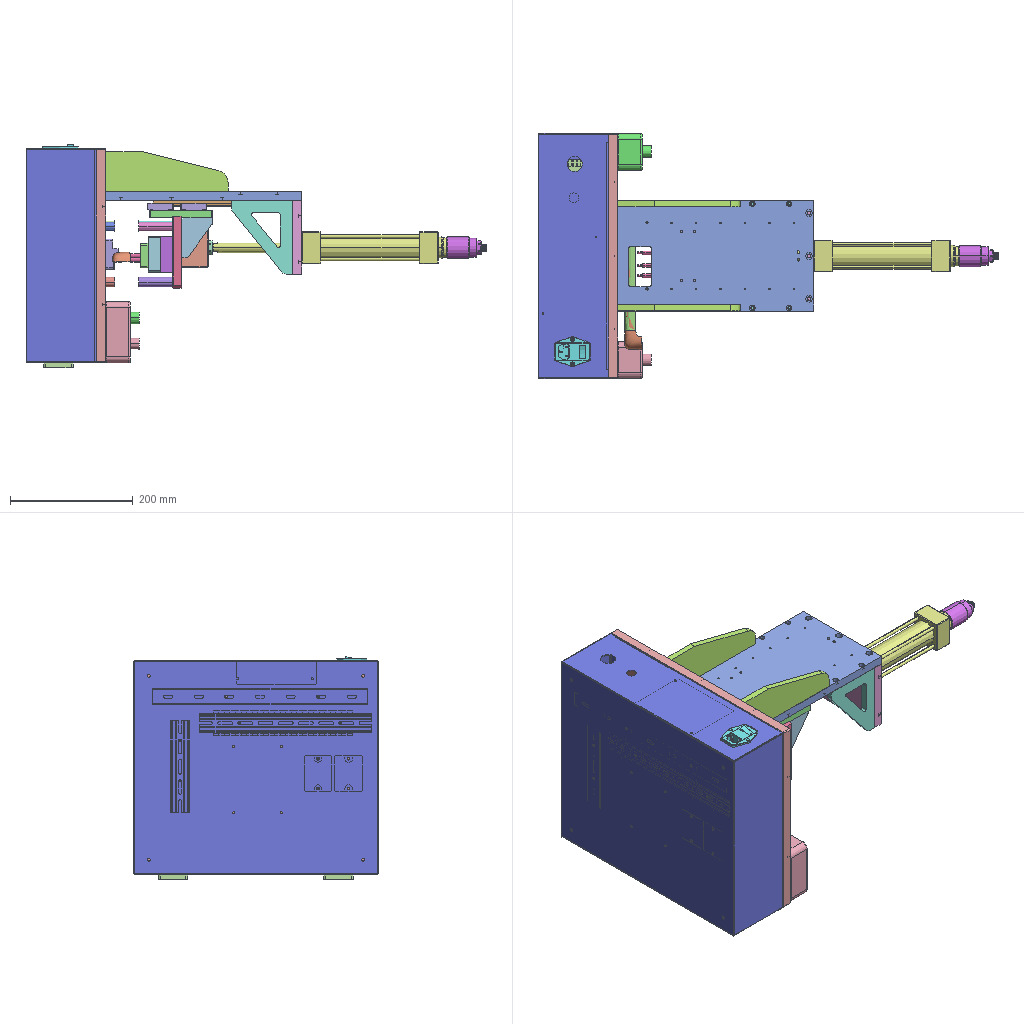Assembly | STEP file | 38 different items | 231 placed | box 751 x 400 x 365 mm
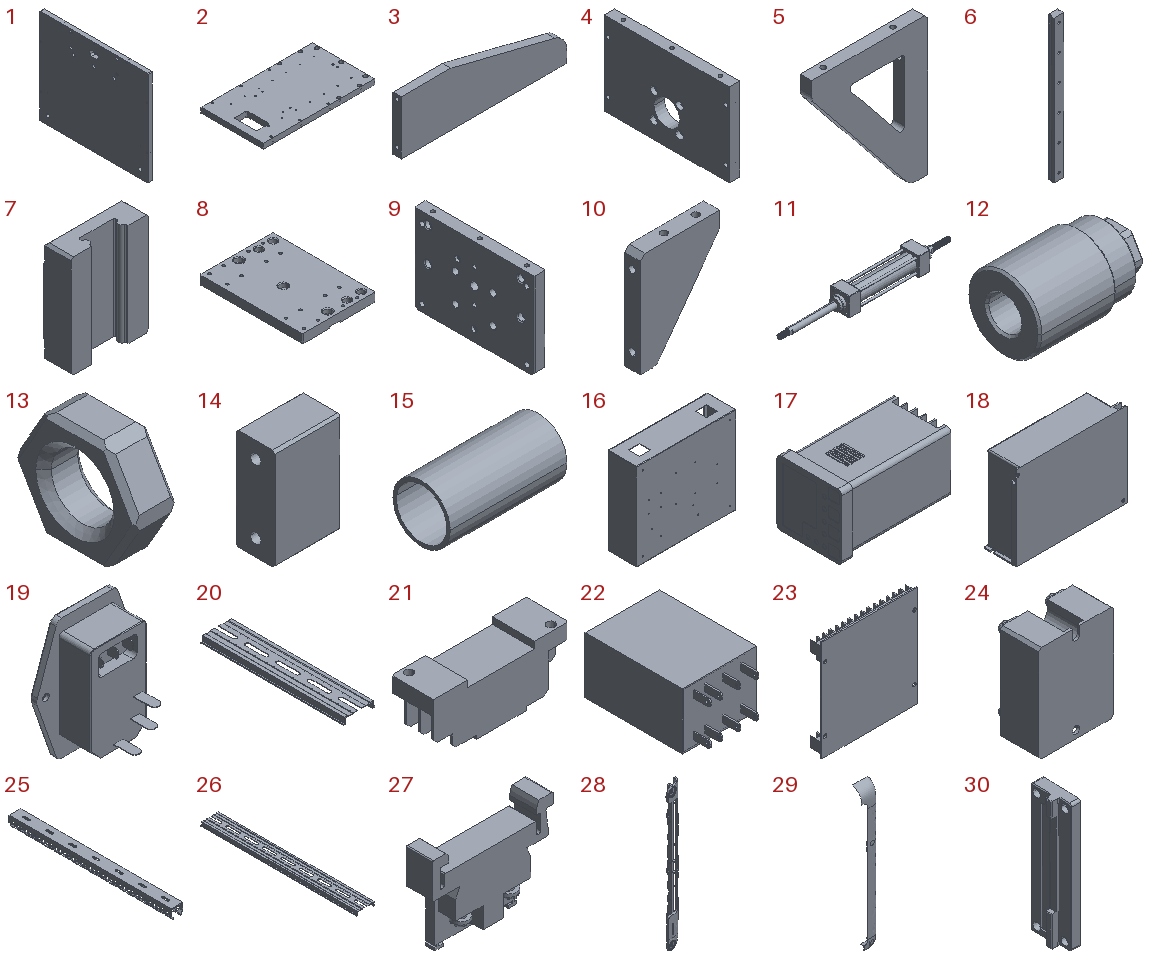Parts list (item | name | quantity | parent item | size | volume):
1 | PN_0002 | x1 | - | 15 x 400 x 350 mm | 2071753 mm3
2 | PN_0003 | x1 | - | 322.5 x 180 x 15 mm | 822668 mm3
3 | PN_0004 | x2 | - | 200 x 10 x 65 mm | 103240 mm3
4 | PN_0005 | x1 | - | 15 x 180 x 120 mm | 300704 mm3
5 | PN_0006 | x2 | - | 100 x 10 x 120 mm | 58710 mm3
6 | PN_0015 | x2 | in Slide rail 16_ASM | 15 x 9.5 x 220 mm | 28688 mm3
7 | PN_0016 | x4 | in Slide rail 16_ASM | 32 x 12 x 42.4 mm | 12345 mm3
8 | PN_0007 | x1 | - | 103 x 145 x 12 mm | 167013 mm3
9 | PN_0008 | x1 | - | 15 x 160 x 117 mm | 266376 mm3
10 | PN_0009 | x2 | - | 50 x 10 x 65 mm | 20426 mm3
11 | PN_0017 | x1 | in Air cylinder 40-125_ASM | 469 x 52 x 52 mm | 443699 mm3
12 | PN_0018 | x1 | in Air cylinder 40-125_ASM | 56 x 35 x 35 mm | 37589 mm3
13 | PN_0019 | x1 | in Air cylinder 40-125_ASM | 8 x 22.5 x 20.785 mm | 1889 mm3
14 | SOLID | x1 | in PN_0010 | 43 x 25 x 65 mm | 61003 mm3
15 | SHELL | x1 | in PN_0010 | - | -
16 | Electrical box 400-350 | x1 | in PN_0001 | 400 x 115 x 350 mm | 480452 mm3
17 | Controller 2 | x2 | in PN_0001 | 83 x 48 x 48 mm | 159214 mm3
18 | Power supply 220-24 | x1 | in PN_0001 | 130 x 37.5 x 98.5 mm | 426318 mm3
19 | Power supply socket base 1 | x1 | in PN_0001 | 48.802 x 32.25 x 59 mm | 19830 mm3
20 | Mounting plate 1 | x1 | in Relay assembly_ASM | 33.46 x 150 x 6.5 mm | 4759 mm3
21 | Fixing bracket 1 | x5 | in Bracket 1_ASM | 71.5 x 22.5 x 29.5 mm | 31610 mm3
22 | Relay 1 | x5 | in Bracket 1_ASM | 26.8 x 41.2 x 20.4 mm | 1978 mm3
23 | Large sheet machine | x1 | in PN_0001 | 116 x 16.2 x 122 mm | 66720 mm3
24 | Solid-state relay 1 | x2 | in PN_0001 | 44.6 x 30 x 57.6 mm | 54499 mm3
25 | Wire tray 25-23 | x1 | in PN_0001 | 25.3 x 350 x 22.5 mm | 27781 mm3
26 | Mounting plate 2 | x1 | in Hot-melt short piece_ASM | 33.46 x 280 x 6.5 mm | 8894 mm3
27 | Short piece 2 | x169 | in Hot-melt short piece_ASM | 41.5 x 9.1 x 33 mm | 6155 mm3
28 | SOLID | x1 | in 111 | 16.497 x 15.143 x 150.563 mm | 2873 mm3
29 | COMPOUND | x1 | in 111 | - | -
30 | 222 | x1 | in Base mould_ASM | 22.319 x 50.323 x 160 mm | 105919 mm3
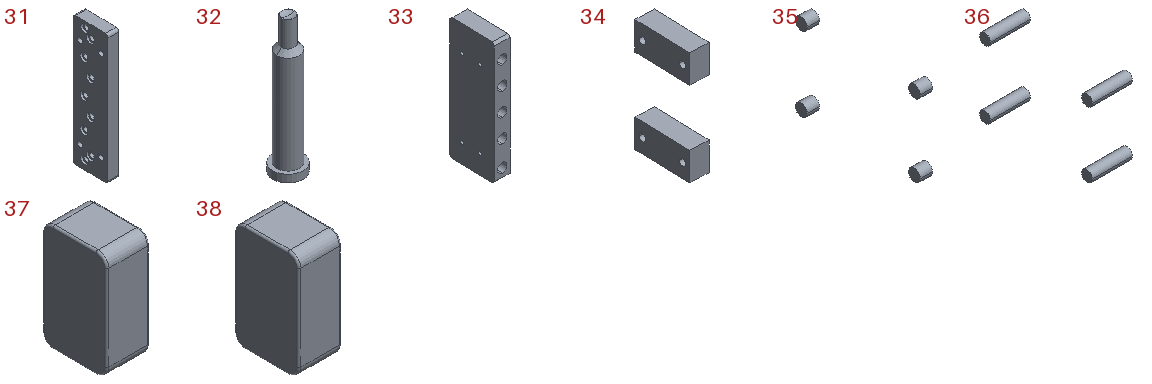31 | 333 | x1 | in Base mould_ASM | 13.043 x 40.3 x 145 mm | 63615 mm3
32 | Hot-melt nozzle | x9 | in Base mould_ASM | 8 x 8 x 36 mm | 921.971 mm3
33 | 555 | x1 | in Base mould_ASM | 21.564 x 60.503 x 160 mm | 156549 mm3
34 | 666 | x1 | in Base mould_ASM | 21.564 x 60.503 x 120 mm | 68921 mm3
35 | PN_0011 | x1 | - | 15 x 155 x 107.5 mm | 10603 mm3
36 | PN_0012 | x1 | - | 55 x 155 x 107.5 mm | 38877 mm3
37 | PN_0013 | x1 | - | 55 x 60 x 100 mm | 243898 mm3
38 | PN_0014 | x1 | - | 55 x 60 x 100 mm | 240255 mm3
Placements (level | parent | child | x y z in mm | rotation matrix by rows):
1 | subassembly 2 | PN_0002 | 0.0 0.0 0.0 | 1 0 0 0 1 0 0 0 1
1 | subassembly 2 | PN_0003 | 0.0 0.0 0.0 | 1 0 0 0 1 0 0 0 1
1 | subassembly 2 | PN_0004 | 0.0 0.0 0.0 | 1 0 0 0 1 0 0 0 1
1 | subassembly 2 | PN_0004 | 0.0 -170.0 0.0 | 1 0 0 0 1 0 0 0 1
1 | subassembly 2 | PN_0005 | 0.0 0.0 0.0 | 1 0 0 0 1 0 0 0 1
1 | subassembly 2 | PN_0006 | 0.0 0.0 0.0 | 1 0 0 0 1 0 0 0 1
1 | subassembly 2 | PN_0006 | 0.0 170.0 0.0 | 1 0 0 0 1 0 0 0 1
1 | subassembly 2 | Slide rail 16_ASM | 93.0 -46.5 80.5 | 0 0 1 -1 0 0 0 -1 0
2 | Slide rail 16_ASM | PN_0015 | 0.0 0.0 0.0 | 1 0 0 0 1 0 0 0 1
2 | Slide rail 16_ASM | PN_0016 | 0.0 0.0 0.0 | 1 0 0 0 1 0 0 0 1
2 | Slide rail 16_ASM | PN_0016 | 15.0 0.0 77.4 | -1 0 0 0 1 0 0 0 -1
1 | subassembly 2 | Slide rail 16_ASM | 93.0 61.5 80.5 | 0 0 1 -1 0 0 0 -1 0
2 | Slide rail 16_ASM | PN_0015 | 0.0 0.0 0.0 | 1 0 0 0 1 0 0 0 1
2 | Slide rail 16_ASM | PN_0016 | 0.0 0.0 0.0 | 1 0 0 0 1 0 0 0 1
2 | Slide rail 16_ASM | PN_0016 | 15.0 0.0 77.4 | -1 0 0 0 1 0 0 0 -1
1 | subassembly 2 | PN_0007 | 0.0 0.0 0.0 | 1 0 0 0 1 0 0 0 1
1 | subassembly 2 | PN_0008 | 0.0 0.0 0.0 | 1 0 0 0 1 0 0 0 1
1 | subassembly 2 | PN_0009 | 0.0 0.0 0.0 | 1 0 0 0 1 0 0 0 1
1 | subassembly 2 | PN_0009 | 0.0 124.0 0.0 | 1 0 0 0 1 0 0 0 1
1 | subassembly 2 | Air cylinder 40-125_ASM | 335.0 0.0 13.0 | 1 0 0 0 1 0 0 0 1
2 | Air cylinder 40-125_ASM | PN_0017 | 0.0 0.0 0.0 | 1 0 0 0 0 1 0 -1 0
2 | Air cylinder 40-125_ASM | PN_0018 | 0.0 0.0 0.0 | 1 0 0 0 0 1 0 -1 0
2 | Air cylinder 40-125_ASM | PN_0019 | 0.0 0.0 0.0 | 1 0 0 0 0 1 0 -1 0
1 | subassembly 2 | PN_0010 | 0.0 0.0 0.0 | 1 0 0 0 1 0 0 0 1
2 | PN_0010 | SOLID | 0.0 0.0 0.0 | 1 0 0 0 1 0 0 0 1
2 | PN_0010 | SHELL | 0.0 0.0 0.0 | 1 0 0 0 1 0 0 0 1
1 | subassembly 2 | PN_0001 | -113.5 0.0 0.0 | 0 1 0 1 0 0 0 0 -1
2 | PN_0001 | Electrical box 400-350 | 0.0 0.0 0.0 | 1 0 0 0 1 0 0 0 1
2 | PN_0001 | Controller 2 | -134.5 51.25 183.0 | 0 0 1 0 1 0 -1 0 0
2 | PN_0001 | Controller 2 | 135.5 51.25 183.0 | 0 0 1 0 1 0 -1 0 0
2 | PN_0001 | Power supply 220-24 | -33.5 50.75 -173.5 | -1 0 0 0 0 1 0 1 0
2 | PN_0001 | Power supply socket base 1 | -156.4 54.7 -175.0 | 1 0 0 0 0 1 0 -1 0
2 | PN_0001 | Relay assembly_ASM | 140.75 0.0 73.5 | -1 0 0 0 0 -1 0 -1 0
3 | Relay assembly_ASM | Mounting plate 1 | 16.73 75.0 5.0 | 1 0 0 0 1 0 0 0 1
3 | Relay assembly_ASM | Bracket 1_ASM | 18.0 26.25 -17.75 | 1 0 0 0 1 0 0 0 1
4 | Bracket 1_ASM | Fixing bracket 1 | 0.0 0.0 0.0 | 1 0 0 0 1 0 0 0 1
4 | Bracket 1_ASM | Relay 1 | 0.0 0.0 -14.85 | -1 0 0 0 0 -1 0 -1 0
3 | Relay assembly_ASM | Bracket 1_ASM | 18.0 51.25 -17.75 | 1 0 0 0 1 0 0 0 1
4 | Bracket 1_ASM | Fixing bracket 1 | 0.0 0.0 0.0 | 1 0 0 0 1 0 0 0 1
4 | Bracket 1_ASM | Relay 1 | 0.0 0.0 -14.85 | -1 0 0 0 0 -1 0 -1 0
3 | Relay assembly_ASM | Bracket 1_ASM | 18.0 76.25 -17.75 | 1 0 0 0 1 0 0 0 1
4 | Bracket 1_ASM | Fixing bracket 1 | 0.0 0.0 0.0 | 1 0 0 0 1 0 0 0 1
4 | Bracket 1_ASM | Relay 1 | 0.0 0.0 -14.85 | -1 0 0 0 0 -1 0 -1 0
3 | Relay assembly_ASM | Bracket 1_ASM | 18.0 101.25 -17.75 | 1 0 0 0 1 0 0 0 1
4 | Bracket 1_ASM | Fixing bracket 1 | 0.0 0.0 0.0 | 1 0 0 0 1 0 0 0 1
4 | Bracket 1_ASM | Relay 1 | 0.0 0.0 -14.85 | -1 0 0 0 0 -1 0 -1 0
3 | Relay assembly_ASM | Bracket 1_ASM | 18.0 126.25 -17.75 | 1 0 0 0 1 0 0 0 1
4 | Bracket 1_ASM | Fixing bracket 1 | 0.0 0.0 0.0 | 1 0 0 0 1 0 0 0 1
4 | Bracket 1_ASM | Relay 1 | 0.0 0.0 -14.85 | -1 0 0 0 0 -1 0 -1 0
2 | PN_0001 | Large sheet machine | -2.5 15.0 19.5 | 0 0 1 0 1 0 -1 0 0
2 | PN_0001 | Solid-state relay 1 | -151.2 0.0 9.7 | 1 0 0 0 1 0 0 0 1
2 | PN_0001 | Solid-state relay 1 | -101.2 0.0 9.7 | 1 0 0 0 1 0 0 0 1
2 | PN_0001 | Wire tray 25-23 | -6.5 10.0 -115.85 | 0 1 0 0 0 -1 -1 0 0
2 | PN_0001 | Hot-melt short piece_ASM | -48.5 -5.0 -72.747 | 0 1 0 0 0 -1 -1 0 0
3 | Hot-melt short piece_ASM | Mounting plate 2 | 0.0 0.0 0.0 | 1 0 0 0 1 0 0 0 1
3 | Hot-melt short piece_ASM | Short piece 2 | 0.0 0.0 -22.2 | 1 0 0 0 1 0 0 0 1
3 | Hot-melt short piece_ASM | Short piece 2 | 0.0 -9.1 -22.2 | 1 0 0 0 1 0 0 0 1
3 | Hot-melt short piece_ASM | Short piece 2 | 0.0 -18.2 -22.2 | 1 0 0 0 1 0 0 0 1
3 | Hot-melt short piece_ASM | Short piece 2 | 0.0 -27.3 -22.2 | 1 0 0 0 1 0 0 0 1
3 | Hot-melt short piece_ASM | Short piece 2 | 0.0 -36.4 -22.2 | 1 0 0 0 1 0 0 0 1
3 | Hot-melt short piece_ASM | Short piece 2 | 0.0 -45.5 -22.2 | 1 0 0 0 1 0 0 0 1
3 | Hot-melt short piece_ASM | Short piece 2 | 0.0 -54.6 -22.2 | 1 0 0 0 1 0 0 0 1
3 | Hot-melt short piece_ASM | Short piece 2 | 0.0 -63.7 -22.2 | 1 0 0 0 1 0 0 0 1
3 | Hot-melt short piece_ASM | Short piece 2 | 0.0 -72.8 -22.2 | 1 0 0 0 1 0 0 0 1
3 | Hot-melt short piece_ASM | Short piece 2 | 0.0 -81.9 -22.2 | 1 0 0 0 1 0 0 0 1
3 | Hot-melt short piece_ASM | Short piece 2 | 0.0 -91.0 -22.2 | 1 0 0 0 1 0 0 0 1
3 | Hot-melt short piece_ASM | Short piece 2 | 0.0 -100.1 -22.2 | 1 0 0 0 1 0 0 0 1
3 | Hot-melt short piece_ASM | Short piece 2 | 0.0 -109.2 -22.2 | 1 0 0 0 1 0 0 0 1
3 | Hot-melt short piece_ASM | Short piece 2 | 0.0 9.1 -22.2 | 1 0 0 0 1 0 0 0 1
3 | Hot-melt short piece_ASM | Short piece 2 | 0.0 0.0 -22.2 | 1 0 0 0 1 0 0 0 1
3 | Hot-melt short piece_ASM | Short piece 2 | 0.0 -9.1 -22.2 | 1 0 0 0 1 0 0 0 1
3 | Hot-melt short piece_ASM | Short piece 2 | 0.0 -18.2 -22.2 | 1 0 0 0 1 0 0 0 1
3 | Hot-melt short piece_ASM | Short piece 2 | 0.0 -27.3 -22.2 | 1 0 0 0 1 0 0 0 1
3 | Hot-melt short piece_ASM | Short piece 2 | 0.0 -36.4 -22.2 | 1 0 0 0 1 0 0 0 1
3 | Hot-melt short piece_ASM | Short piece 2 | 0.0 -45.5 -22.2 | 1 0 0 0 1 0 0 0 1
3 | Hot-melt short piece_ASM | Short piece 2 | 0.0 -54.6 -22.2 | 1 0 0 0 1 0 0 0 1
3 | Hot-melt short piece_ASM | Short piece 2 | 0.0 -63.7 -22.2 | 1 0 0 0 1 0 0 0 1
3 | Hot-melt short piece_ASM | Short piece 2 | 0.0 -72.8 -22.2 | 1 0 0 0 1 0 0 0 1
3 | Hot-melt short piece_ASM | Short piece 2 | 0.0 -81.9 -22.2 | 1 0 0 0 1 0 0 0 1
3 | Hot-melt short piece_ASM | Short piece 2 | 0.0 -91.0 -22.2 | 1 0 0 0 1 0 0 0 1
3 | Hot-melt short piece_ASM | Short piece 2 | 0.0 -100.1 -22.2 | 1 0 0 0 1 0 0 0 1
3 | Hot-melt short piece_ASM | Short piece 2 | 0.0 18.2 -22.2 | 1 0 0 0 1 0 0 0 1
3 | Hot-melt short piece_ASM | Short piece 2 | 0.0 9.1 -22.2 | 1 0 0 0 1 0 0 0 1
3 | Hot-melt short piece_ASM | Short piece 2 | 0.0 0.0 -22.2 | 1 0 0 0 1 0 0 0 1
3 | Hot-melt short piece_ASM | Short piece 2 | 0.0 -9.1 -22.2 | 1 0 0 0 1 0 0 0 1
3 | Hot-melt short piece_ASM | Short piece 2 | 0.0 -18.2 -22.2 | 1 0 0 0 1 0 0 0 1
3 | Hot-melt short piece_ASM | Short piece 2 | 0.0 -27.3 -22.2 | 1 0 0 0 1 0 0 0 1
3 | Hot-melt short piece_ASM | Short piece 2 | 0.0 -36.4 -22.2 | 1 0 0 0 1 0 0 0 1
3 | Hot-melt short piece_ASM | Short piece 2 | 0.0 -45.5 -22.2 | 1 0 0 0 1 0 0 0 1
3 | Hot-melt short piece_ASM | Short piece 2 | 0.0 -54.6 -22.2 | 1 0 0 0 1 0 0 0 1
3 | Hot-melt short piece_ASM | Short piece 2 | 0.0 -63.7 -22.2 | 1 0 0 0 1 0 0 0 1
3 | Hot-melt short piece_ASM | Short piece 2 | 0.0 -72.8 -22.2 | 1 0 0 0 1 0 0 0 1
3 | Hot-melt short piece_ASM | Short piece 2 | 0.0 -81.9 -22.2 | 1 0 0 0 1 0 0 0 1
3 | Hot-melt short piece_ASM | Short piece 2 | 0.0 -91.0 -22.2 | 1 0 0 0 1 0 0 0 1
3 | Hot-melt short piece_ASM | Short piece 2 | 0.0 27.3 -22.2 | 1 0 0 0 1 0 0 0 1
3 | Hot-melt short piece_ASM | Short piece 2 | 0.0 18.2 -22.2 | 1 0 0 0 1 0 0 0 1
3 | Hot-melt short piece_ASM | Short piece 2 | 0.0 9.1 -22.2 | 1 0 0 0 1 0 0 0 1
3 | Hot-melt short piece_ASM | Short piece 2 | 0.0 0.0 -22.2 | 1 0 0 0 1 0 0 0 1
3 | Hot-melt short piece_ASM | Short piece 2 | 0.0 -9.1 -22.2 | 1 0 0 0 1 0 0 0 1
3 | Hot-melt short piece_ASM | Short piece 2 | 0.0 -18.2 -22.2 | 1 0 0 0 1 0 0 0 1
3 | Hot-melt short piece_ASM | Short piece 2 | 0.0 -27.3 -22.2 | 1 0 0 0 1 0 0 0 1
3 | Hot-melt short piece_ASM | Short piece 2 | 0.0 -36.4 -22.2 | 1 0 0 0 1 0 0 0 1
3 | Hot-melt short piece_ASM | Short piece 2 | 0.0 -45.5 -22.2 | 1 0 0 0 1 0 0 0 1
3 | Hot-melt short piece_ASM | Short piece 2 | 0.0 -54.6 -22.2 | 1 0 0 0 1 0 0 0 1
3 | Hot-melt short piece_ASM | Short piece 2 | 0.0 -63.7 -22.2 | 1 0 0 0 1 0 0 0 1
3 | Hot-melt short piece_ASM | Short piece 2 | 0.0 -72.8 -22.2 | 1 0 0 0 1 0 0 0 1
3 | Hot-melt short piece_ASM | Short piece 2 | 0.0 -81.9 -22.2 | 1 0 0 0 1 0 0 0 1
3 | Hot-melt short piece_ASM | Short piece 2 | 0.0 36.4 -22.2 | 1 0 0 0 1 0 0 0 1
3 | Hot-melt short piece_ASM | Short piece 2 | 0.0 27.3 -22.2 | 1 0 0 0 1 0 0 0 1
3 | Hot-melt short piece_ASM | Short piece 2 | 0.0 18.2 -22.2 | 1 0 0 0 1 0 0 0 1
3 | Hot-melt short piece_ASM | Short piece 2 | 0.0 9.1 -22.2 | 1 0 0 0 1 0 0 0 1
3 | Hot-melt short piece_ASM | Short piece 2 | 0.0 0.0 -22.2 | 1 0 0 0 1 0 0 0 1
3 | Hot-melt short piece_ASM | Short piece 2 | 0.0 -9.1 -22.2 | 1 0 0 0 1 0 0 0 1
3 | Hot-melt short piece_ASM | Short piece 2 | 0.0 -18.2 -22.2 | 1 0 0 0 1 0 0 0 1
3 | Hot-melt short piece_ASM | Short piece 2 | 0.0 -27.3 -22.2 | 1 0 0 0 1 0 0 0 1
3 | Hot-melt short piece_ASM | Short piece 2 | 0.0 -36.4 -22.2 | 1 0 0 0 1 0 0 0 1
3 | Hot-melt short piece_ASM | Short piece 2 | 0.0 -45.5 -22.2 | 1 0 0 0 1 0 0 0 1
3 | Hot-melt short piece_ASM | Short piece 2 | 0.0 -54.6 -22.2 | 1 0 0 0 1 0 0 0 1
3 | Hot-melt short piece_ASM | Short piece 2 | 0.0 -63.7 -22.2 | 1 0 0 0 1 0 0 0 1
3 | Hot-melt short piece_ASM | Short piece 2 | 0.0 -72.8 -22.2 | 1 0 0 0 1 0 0 0 1
3 | Hot-melt short piece_ASM | Short piece 2 | 0.0 45.5 -22.2 | 1 0 0 0 1 0 0 0 1
3 | Hot-melt short piece_ASM | Short piece 2 | 0.0 36.4 -22.2 | 1 0 0 0 1 0 0 0 1
3 | Hot-melt short piece_ASM | Short piece 2 | 0.0 27.3 -22.2 | 1 0 0 0 1 0 0 0 1
3 | Hot-melt short piece_ASM | Short piece 2 | 0.0 18.2 -22.2 | 1 0 0 0 1 0 0 0 1
3 | Hot-melt short piece_ASM | Short piece 2 | 0.0 9.1 -22.2 | 1 0 0 0 1 0 0 0 1
3 | Hot-melt short piece_ASM | Short piece 2 | 0.0 0.0 -22.2 | 1 0 0 0 1 0 0 0 1
3 | Hot-melt short piece_ASM | Short piece 2 | 0.0 -9.1 -22.2 | 1 0 0 0 1 0 0 0 1
3 | Hot-melt short piece_ASM | Short piece 2 | 0.0 -18.2 -22.2 | 1 0 0 0 1 0 0 0 1
3 | Hot-melt short piece_ASM | Short piece 2 | 0.0 -27.3 -22.2 | 1 0 0 0 1 0 0 0 1
3 | Hot-melt short piece_ASM | Short piece 2 | 0.0 -36.4 -22.2 | 1 0 0 0 1 0 0 0 1
3 | Hot-melt short piece_ASM | Short piece 2 | 0.0 -45.5 -22.2 | 1 0 0 0 1 0 0 0 1
3 | Hot-melt short piece_ASM | Short piece 2 | 0.0 -54.6 -22.2 | 1 0 0 0 1 0 0 0 1
3 | Hot-melt short piece_ASM | Short piece 2 | 0.0 -63.7 -22.2 | 1 0 0 0 1 0 0 0 1
3 | Hot-melt short piece_ASM | Short piece 2 | 0.0 54.6 -22.2 | 1 0 0 0 1 0 0 0 1
3 | Hot-melt short piece_ASM | Short piece 2 | 0.0 45.5 -22.2 | 1 0 0 0 1 0 0 0 1
3 | Hot-melt short piece_ASM | Short piece 2 | 0.0 36.4 -22.2 | 1 0 0 0 1 0 0 0 1
3 | Hot-melt short piece_ASM | Short piece 2 | 0.0 27.3 -22.2 | 1 0 0 0 1 0 0 0 1
3 | Hot-melt short piece_ASM | Short piece 2 | 0.0 18.2 -22.2 | 1 0 0 0 1 0 0 0 1
3 | Hot-melt short piece_ASM | Short piece 2 | 0.0 9.1 -22.2 | 1 0 0 0 1 0 0 0 1
3 | Hot-melt short piece_ASM | Short piece 2 | 0.0 0.0 -22.2 | 1 0 0 0 1 0 0 0 1
3 | Hot-melt short piece_ASM | Short piece 2 | 0.0 -9.1 -22.2 | 1 0 0 0 1 0 0 0 1
3 | Hot-melt short piece_ASM | Short piece 2 | 0.0 -18.2 -22.2 | 1 0 0 0 1 0 0 0 1
3 | Hot-melt short piece_ASM | Short piece 2 | 0.0 -27.3 -22.2 | 1 0 0 0 1 0 0 0 1
3 | Hot-melt short piece_ASM | Short piece 2 | 0.0 -36.4 -22.2 | 1 0 0 0 1 0 0 0 1
3 | Hot-melt short piece_ASM | Short piece 2 | 0.0 -45.5 -22.2 | 1 0 0 0 1 0 0 0 1
3 | Hot-melt short piece_ASM | Short piece 2 | 0.0 -54.6 -22.2 | 1 0 0 0 1 0 0 0 1
3 | Hot-melt short piece_ASM | Short piece 2 | 0.0 63.7 -22.2 | 1 0 0 0 1 0 0 0 1
3 | Hot-melt short piece_ASM | Short piece 2 | 0.0 54.6 -22.2 | 1 0 0 0 1 0 0 0 1
3 | Hot-melt short piece_ASM | Short piece 2 | 0.0 45.5 -22.2 | 1 0 0 0 1 0 0 0 1
3 | Hot-melt short piece_ASM | Short piece 2 | 0.0 36.4 -22.2 | 1 0 0 0 1 0 0 0 1
3 | Hot-melt short piece_ASM | Short piece 2 | 0.0 27.3 -22.2 | 1 0 0 0 1 0 0 0 1
3 | Hot-melt short piece_ASM | Short piece 2 | 0.0 18.2 -22.2 | 1 0 0 0 1 0 0 0 1
3 | Hot-melt short piece_ASM | Short piece 2 | 0.0 9.1 -22.2 | 1 0 0 0 1 0 0 0 1
3 | Hot-melt short piece_ASM | Short piece 2 | 0.0 0.0 -22.2 | 1 0 0 0 1 0 0 0 1
3 | Hot-melt short piece_ASM | Short piece 2 | 0.0 -9.1 -22.2 | 1 0 0 0 1 0 0 0 1
3 | Hot-melt short piece_ASM | Short piece 2 | 0.0 -18.2 -22.2 | 1 0 0 0 1 0 0 0 1
3 | Hot-melt short piece_ASM | Short piece 2 | 0.0 -27.3 -22.2 | 1 0 0 0 1 0 0 0 1
3 | Hot-melt short piece_ASM | Short piece 2 | 0.0 -36.4 -22.2 | 1 0 0 0 1 0 0 0 1
3 | Hot-melt short piece_ASM | Short piece 2 | 0.0 -45.5 -22.2 | 1 0 0 0 1 0 0 0 1
3 | Hot-melt short piece_ASM | Short piece 2 | 0.0 72.8 -22.2 | 1 0 0 0 1 0 0 0 1
3 | Hot-melt short piece_ASM | Short piece 2 | 0.0 63.7 -22.2 | 1 0 0 0 1 0 0 0 1
3 | Hot-melt short piece_ASM | Short piece 2 | 0.0 54.6 -22.2 | 1 0 0 0 1 0 0 0 1
3 | Hot-melt short piece_ASM | Short piece 2 | 0.0 45.5 -22.2 | 1 0 0 0 1 0 0 0 1
3 | Hot-melt short piece_ASM | Short piece 2 | 0.0 36.4 -22.2 | 1 0 0 0 1 0 0 0 1
3 | Hot-melt short piece_ASM | Short piece 2 | 0.0 27.3 -22.2 | 1 0 0 0 1 0 0 0 1
3 | Hot-melt short piece_ASM | Short piece 2 | 0.0 18.2 -22.2 | 1 0 0 0 1 0 0 0 1
3 | Hot-melt short piece_ASM | Short piece 2 | 0.0 9.1 -22.2 | 1 0 0 0 1 0 0 0 1
3 | Hot-melt short piece_ASM | Short piece 2 | 0.0 0.0 -22.2 | 1 0 0 0 1 0 0 0 1
3 | Hot-melt short piece_ASM | Short piece 2 | 0.0 -9.1 -22.2 | 1 0 0 0 1 0 0 0 1
3 | Hot-melt short piece_ASM | Short piece 2 | 0.0 -18.2 -22.2 | 1 0 0 0 1 0 0 0 1
3 | Hot-melt short piece_ASM | Short piece 2 | 0.0 -27.3 -22.2 | 1 0 0 0 1 0 0 0 1
3 | Hot-melt short piece_ASM | Short piece 2 | 0.0 -36.4 -22.2 | 1 0 0 0 1 0 0 0 1
3 | Hot-melt short piece_ASM | Short piece 2 | 0.0 81.9 -22.2 | 1 0 0 0 1 0 0 0 1
3 | Hot-melt short piece_ASM | Short piece 2 | 0.0 72.8 -22.2 | 1 0 0 0 1 0 0 0 1
3 | Hot-melt short piece_ASM | Short piece 2 | 0.0 63.7 -22.2 | 1 0 0 0 1 0 0 0 1
3 | Hot-melt short piece_ASM | Short piece 2 | 0.0 54.6 -22.2 | 1 0 0 0 1 0 0 0 1
3 | Hot-melt short piece_ASM | Short piece 2 | 0.0 45.5 -22.2 | 1 0 0 0 1 0 0 0 1
3 | Hot-melt short piece_ASM | Short piece 2 | 0.0 36.4 -22.2 | 1 0 0 0 1 0 0 0 1
3 | Hot-melt short piece_ASM | Short piece 2 | 0.0 27.3 -22.2 | 1 0 0 0 1 0 0 0 1
3 | Hot-melt short piece_ASM | Short piece 2 | 0.0 18.2 -22.2 | 1 0 0 0 1 0 0 0 1
3 | Hot-melt short piece_ASM | Short piece 2 | 0.0 9.1 -22.2 | 1 0 0 0 1 0 0 0 1
3 | Hot-melt short piece_ASM | Short piece 2 | 0.0 0.0 -22.2 | 1 0 0 0 1 0 0 0 1
3 | Hot-melt short piece_ASM | Short piece 2 | 0.0 -9.1 -22.2 | 1 0 0 0 1 0 0 0 1
3 | Hot-melt short piece_ASM | Short piece 2 | 0.0 -18.2 -22.2 | 1 0 0 0 1 0 0 0 1
3 | Hot-melt short piece_ASM | Short piece 2 | 0.0 -27.3 -22.2 | 1 0 0 0 1 0 0 0 1
3 | Hot-melt short piece_ASM | Short piece 2 | 0.0 91.0 -22.2 | 1 0 0 0 1 0 0 0 1
3 | Hot-melt short piece_ASM | Short piece 2 | 0.0 81.9 -22.2 | 1 0 0 0 1 0 0 0 1
3 | Hot-melt short piece_ASM | Short piece 2 | 0.0 72.8 -22.2 | 1 0 0 0 1 0 0 0 1
3 | Hot-melt short piece_ASM | Short piece 2 | 0.0 63.7 -22.2 | 1 0 0 0 1 0 0 0 1
3 | Hot-melt short piece_ASM | Short piece 2 | 0.0 54.6 -22.2 | 1 0 0 0 1 0 0 0 1
3 | Hot-melt short piece_ASM | Short piece 2 | 0.0 45.5 -22.2 | 1 0 0 0 1 0 0 0 1
3 | Hot-melt short piece_ASM | Short piece 2 | 0.0 36.4 -22.2 | 1 0 0 0 1 0 0 0 1
3 | Hot-melt short piece_ASM | Short piece 2 | 0.0 27.3 -22.2 | 1 0 0 0 1 0 0 0 1
3 | Hot-melt short piece_ASM | Short piece 2 | 0.0 18.2 -22.2 | 1 0 0 0 1 0 0 0 1
3 | Hot-melt short piece_ASM | Short piece 2 | 0.0 9.1 -22.2 | 1 0 0 0 1 0 0 0 1
3 | Hot-melt short piece_ASM | Short piece 2 | 0.0 0.0 -22.2 | 1 0 0 0 1 0 0 0 1
3 | Hot-melt short piece_ASM | Short piece 2 | 0.0 -9.1 -22.2 | 1 0 0 0 1 0 0 0 1
3 | Hot-melt short piece_ASM | Short piece 2 | 0.0 -18.2 -22.2 | 1 0 0 0 1 0 0 0 1
3 | Hot-melt short piece_ASM | Short piece 2 | 0.0 100.1 -22.2 | 1 0 0 0 1 0 0 0 1
3 | Hot-melt short piece_ASM | Short piece 2 | 0.0 91.0 -22.2 | 1 0 0 0 1 0 0 0 1
3 | Hot-melt short piece_ASM | Short piece 2 | 0.0 81.9 -22.2 | 1 0 0 0 1 0 0 0 1
3 | Hot-melt short piece_ASM | Short piece 2 | 0.0 72.8 -22.2 | 1 0 0 0 1 0 0 0 1
3 | Hot-melt short piece_ASM | Short piece 2 | 0.0 63.7 -22.2 | 1 0 0 0 1 0 0 0 1
3 | Hot-melt short piece_ASM | Short piece 2 | 0.0 54.6 -22.2 | 1 0 0 0 1 0 0 0 1
3 | Hot-melt short piece_ASM | Short piece 2 | 0.0 45.5 -22.2 | 1 0 0 0 1 0 0 0 1
3 | Hot-melt short piece_ASM | Short piece 2 | 0.0 36.4 -22.2 | 1 0 0 0 1 0 0 0 1
3 | Hot-melt short piece_ASM | Short piece 2 | 0.0 27.3 -22.2 | 1 0 0 0 1 0 0 0 1
3 | Hot-melt short piece_ASM | Short piece 2 | 0.0 18.2 -22.2 | 1 0 0 0 1 0 0 0 1
3 | Hot-melt short piece_ASM | Short piece 2 | 0.0 9.1 -22.2 | 1 0 0 0 1 0 0 0 1
3 | Hot-melt short piece_ASM | Short piece 2 | 0.0 0.0 -22.2 | 1 0 0 0 1 0 0 0 1
3 | Hot-melt short piece_ASM | Short piece 2 | 0.0 -9.1 -22.2 | 1 0 0 0 1 0 0 0 1
3 | Hot-melt short piece_ASM | Short piece 2 | 0.0 109.2 -22.2 | 1 0 0 0 1 0 0 0 1
3 | Hot-melt short piece_ASM | Short piece 2 | 0.0 100.1 -22.2 | 1 0 0 0 1 0 0 0 1
3 | Hot-melt short piece_ASM | Short piece 2 | 0.0 91.0 -22.2 | 1 0 0 0 1 0 0 0 1
3 | Hot-melt short piece_ASM | Short piece 2 | 0.0 81.9 -22.2 | 1 0 0 0 1 0 0 0 1
3 | Hot-melt short piece_ASM | Short piece 2 | 0.0 72.8 -22.2 | 1 0 0 0 1 0 0 0 1
3 | Hot-melt short piece_ASM | Short piece 2 | 0.0 63.7 -22.2 | 1 0 0 0 1 0 0 0 1
3 | Hot-melt short piece_ASM | Short piece 2 | 0.0 54.6 -22.2 | 1 0 0 0 1 0 0 0 1
3 | Hot-melt short piece_ASM | Short piece 2 | 0.0 45.5 -22.2 | 1 0 0 0 1 0 0 0 1
3 | Hot-melt short piece_ASM | Short piece 2 | 0.0 36.4 -22.2 | 1 0 0 0 1 0 0 0 1
3 | Hot-melt short piece_ASM | Short piece 2 | 0.0 27.3 -22.2 | 1 0 0 0 1 0 0 0 1
3 | Hot-melt short piece_ASM | Short piece 2 | 0.0 18.2 -22.2 | 1 0 0 0 1 0 0 0 1
3 | Hot-melt short piece_ASM | Short piece 2 | 0.0 9.1 -22.2 | 1 0 0 0 1 0 0 0 1
3 | Hot-melt short piece_ASM | Short piece 2 | 0.0 0.0 -22.2 | 1 0 0 0 1 0 0 0 1
1 | subassembly 2 | Base mould_ASM | 192.593 80.0 -7.716 | -0.9997 0.02618 0 0 0 -1 -0.02618 -0.9997 0
2 | Base mould_ASM | 111 | 0.0 0.0 0.0 | 1 0 0 0 1 0 0 0 1
3 | 111 | SOLID | 0.0 0.0 0.0 | 1 0 0 0 1 0 0 0 1
3 | 111 | COMPOUND | 0.0 0.0 0.0 | 1 0 0 0 1 0 0 0 1
2 | Base mould_ASM | 222 | 0.0 0.0 0.0 | 1 0 0 0 1 0 0 0 1
2 | Base mould_ASM | 333 | 0.0 0.0 0.0 | 1 0 0 0 1 0 0 0 1
2 | Base mould_ASM | Hot-melt nozzle | 145.257 -148.451 305.4 | 0.02618 0 0.9997 0.9997 0 -0.02618 0 1 0
2 | Base mould_ASM | Hot-melt nozzle | 145.087 -154.938 298.4 | 0.02618 0 0.9997 0.9997 0 -0.02618 0 1 0
2 | Base mould_ASM | Hot-melt nozzle | 145.275 -147.751 276.9 | 0.02618 0 0.9997 0.9997 0 -0.02618 0 1 0
2 | Base mould_ASM | Hot-melt nozzle | 145.087 -154.938 260.232 | 0.02618 0 0.9997 0.9997 0 -0.02618 0 1 0
2 | Base mould_ASM | Hot-melt nozzle | 145.275 -147.751 239.4 | 0.02618 0 0.9997 0.9997 0 -0.02618 0 1 0
2 | Base mould_ASM | Hot-melt nozzle | 145.087 -154.938 222.4 | 0.02618 0 0.9997 0.9997 0 -0.02618 0 1 0
2 | Base mould_ASM | Hot-melt nozzle | 145.276 -147.743 205.9 | 0.02618 0 0.9997 0.9997 0 -0.02618 0 1 0
2 | Base mould_ASM | Hot-melt nozzle | 145.087 -154.946 184.4 | 0.02618 0 0.9997 0.9997 0 -0.02618 0 1 0
2 | Base mould_ASM | Hot-melt nozzle | 145.257 -148.451 177.4 | 0.02618 0 0.9997 0.9997 0 -0.02618 0 1 0
2 | Base mould_ASM | 555 | 0.0 0.0 0.0 | 1 0 0 0 1 0 0 0 1
2 | Base mould_ASM | 666 | 0.0 0.0 0.0 | 1 0 0 0 1 0 0 0 1
1 | subassembly 2 | PN_0011 | 0.0 0.0 0.0 | 1 0 0 0 1 0 0 0 1
1 | subassembly 2 | PN_0012 | 0.0 0.0 0.0 | 1 0 0 0 1 0 0 0 1
1 | subassembly 2 | PN_0013 | 0.0 0.0 0.0 | 1 0 0 0 1 0 0 0 1
1 | subassembly 2 | PN_0014 | 0.0 -340.0 -0.0 | 1 0 0 0 1 0 0 0 1